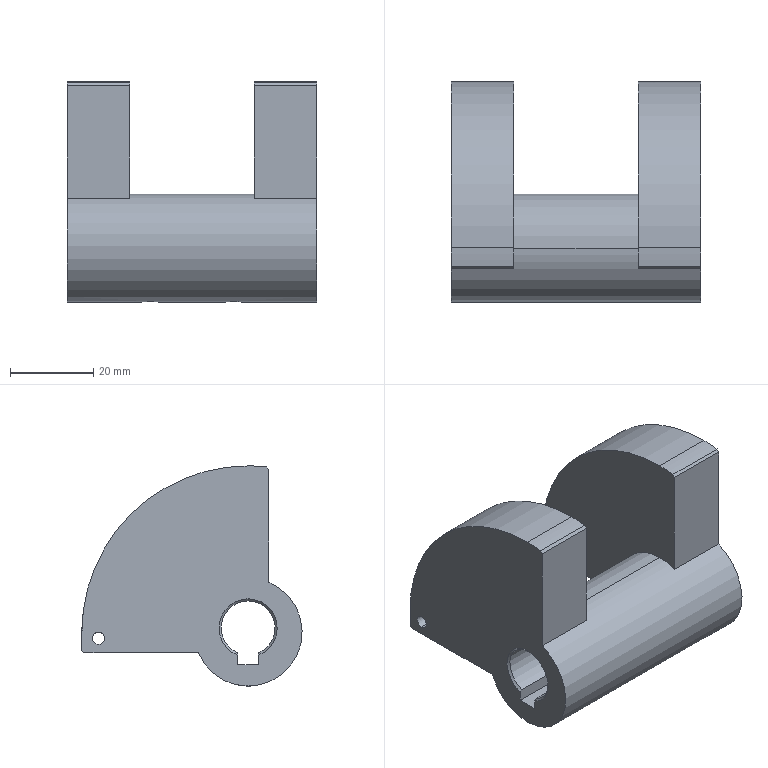Part | SolidWorks | features ICE 5, Chamfer 2, Extrusion 1, HoleWzd 1 | 1 solid | 53 faces | box 60 x 53 x 53 mm | volume 64620 mm3 | cylinder 27 | plane 19 | cone 5 | spline 2 | commonest cylinder face diameters 3 x16 4.2 x4 80 x4 26 x2 13 x1